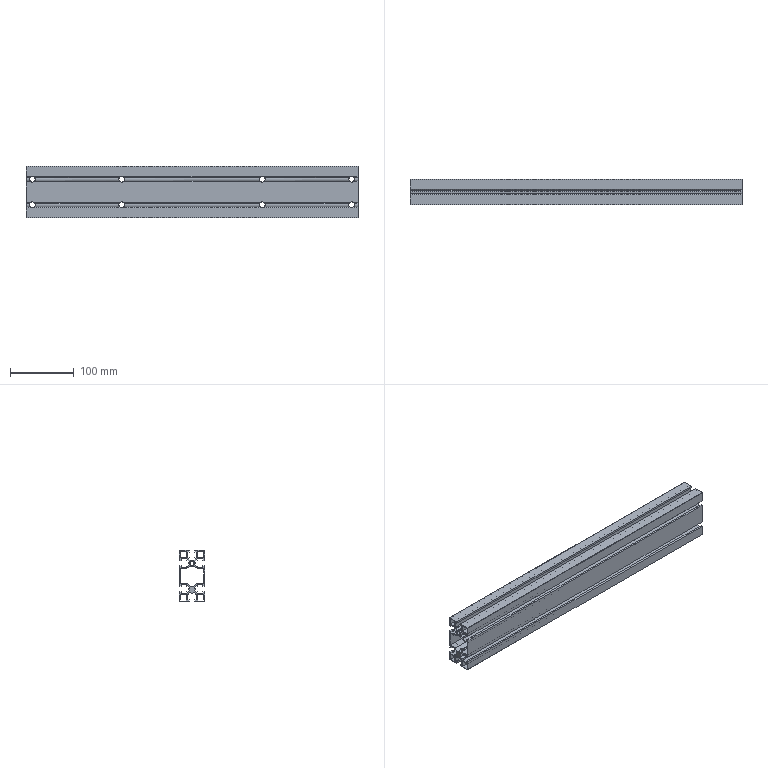Part | STEP file | 1 solid | 330 faces | box 520 x 40 x 80 mm | volume 378549 mm3 | plane 170 | cylinder 160 | commonest cylinder face diameters 9 x76 15 x38 9.6 x33 6.6 x10 0.6 x2 13.3 x1